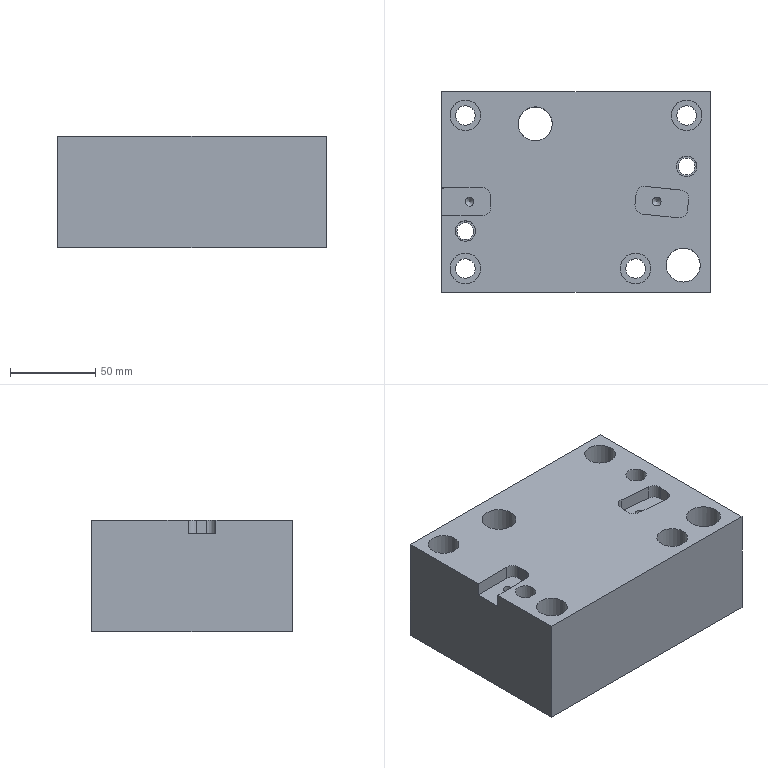Part | NX | features 23 2 | 1 solid | 45 faces | box 158 x 118 x 65.4 mm | volume 1108387 mm3 | cylinder 22 | plane 21 | cone 2 | commonest cylinder face diameters 10 x6 11.5 x4 18 x4 5.2 x2 10.001 x2 12 x2
STEP:
#1=CARTESIAN_POINT('',(1768.,-262.,2.4));
#2=VERTEX_POINT('',#1);
#3=CARTESIAN_POINT('',(1759.,-262.,2.4));
#4=DIRECTION('',(0.,0.,-1.));
#5=DIRECTION('',(1.,0.,0.));
#6=AXIS2_PLACEMENT_3D('',#3,#4,#5);
#7=CIRCLE('',#6,9.);
#8=EDGE_CURVE('',#2,#2,#7,.T.);
#9=ORIENTED_EDGE('',*,*,#8,.T.);
#10=EDGE_LOOP('',(#9));
#11=FACE_BOUND('',#10,.T.);
#12=CARTESIAN_POINT('',(1757.,-340.,2.4));
#13=VERTEX_POINT('',#12);
#14=CARTESIAN_POINT('',(1757.,-350.,2.4));
#15=DIRECTION('',(0.,-0.000000004,1.));
#16=DIRECTION('',(0.,1.,0.000000004));
#17=AXIS2_PLACEMENT_3D('',#14,#15,#16);
#18=CIRCLE('',#17,10.);
#19=EDGE_CURVE('',#13,#13,#18,.T.);
#20=ORIENTED_EDGE('',*,*,#19,.F.);
#21=EDGE_LOOP('',(#20));
#22=FACE_BOUND('',#21,.T.);
#23=CARTESIAN_POINT('',(1728.677,-314.602,2.4));
#24=VERTEX_POINT('',#23);
#25=CARTESIAN_POINT('',(1729.324,-308.234,2.4));
#26=VERTEX_POINT('',#25);
#27=CARTESIAN_POINT('',(1741.75,-185.905,2.4));
#28=DIRECTION('',(0.1011,0.9949,0.000000004));
#29=VECTOR('',#28,1000.);
#30=LINE('',#27,#29);
#31=EDGE_CURVE('',#24,#26,#30,.T.);
#32=ORIENTED_EDGE('',*,*,#31,.T.);
#33=CARTESIAN_POINT('',(1734.804,-303.765,2.4));
#34=VERTEX_POINT('',#33);
#35=CARTESIAN_POINT('',(1734.299,-308.74,2.4));
#36=DIRECTION('',(0.,0.000000004,-1.));
#37=DIRECTION('',(0.,1.,0.000000004));
#38=AXIS2_PLACEMENT_3D('',#35,#36,#37);
#39=CIRCLE('',#38,5.);
#40=EDGE_CURVE('',#26,#34,#39,.T.);
#41=ORIENTED_EDGE('',*,*,#40,.T.);
#42=CARTESIAN_POINT('',(1755.696,-305.887,2.4));
#43=VERTEX_POINT('',#42);
#44=CARTESIAN_POINT('',(1711.08,-301.355,2.4));
#45=DIRECTION('',(0.9949,-0.1011,0.));
#46=VECTOR('',#45,1000.);
#47=LINE('',#44,#46);
#48=EDGE_CURVE('',#34,#43,#47,.T.);
#49=ORIENTED_EDGE('',*,*,#48,.T.);
#50=CARTESIAN_POINT('',(1760.166,-311.367,2.4));
#51=VERTEX_POINT('',#50);
#52=CARTESIAN_POINT('',(1755.191,-310.862,2.4));
#53=DIRECTION('',(0.,0.000000004,-1.));
#54=DIRECTION('',(0.,1.,0.000000004));
#55=AXIS2_PLACEMENT_3D('',#52,#53,#54);
#56=CIRCLE('',#55,5.);
#57=EDGE_CURVE('',#43,#51,#56,.T.);
#58=ORIENTED_EDGE('',*,*,#57,.T.);
#59=CARTESIAN_POINT('',(1759.519,-317.734,2.4));
#60=VERTEX_POINT('',#59);
#61=CARTESIAN_POINT('',(1772.591,-189.037,2.4));
#62=DIRECTION('',(-0.1011,-0.9949,-0.000000004));
#63=VECTOR('',#62,1000.);
#64=LINE('',#61,#63);
#65=EDGE_CURVE('',#51,#60,#64,.T.);
#66=ORIENTED_EDGE('',*,*,#65,.T.);
#67=CARTESIAN_POINT('',(1754.039,-322.203,2.4));
#68=VERTEX_POINT('',#67);
#69=CARTESIAN_POINT('',(1754.544,-317.229,2.4));
#70=DIRECTION('',(0.,0.000000004,-1.));
#71=DIRECTION('',(0.,1.,0.000000004));
#72=AXIS2_PLACEMENT_3D('',#69,#70,#71);
#73=CIRCLE('',#72,5.);
#74=EDGE_CURVE('',#60,#68,#73,.T.);
#75=ORIENTED_EDGE('',*,*,#74,.T.);
#76=CARTESIAN_POINT('',(1733.147,-320.081,2.4));
#77=VERTEX_POINT('',#76);
#78=CARTESIAN_POINT('',(1709.422,-317.671,2.4));
#79=DIRECTION('',(-0.9949,0.1011,0.));
#80=VECTOR('',#79,1000.);
#81=LINE('',#78,#80);
#82=EDGE_CURVE('',#68,#77,#81,.T.);
#83=ORIENTED_EDGE('',*,*,#82,.T.);
#84=CARTESIAN_POINT('',(1733.652,-315.107,2.4));
#85=DIRECTION('',(0.,0.000000004,-1.));
#86=DIRECTION('',(0.,1.,0.000000004));
#87=AXIS2_PLACEMENT_3D('',#84,#85,#86);
#88=CIRCLE('',#87,5.);
#89=EDGE_CURVE('',#77,#24,#88,.T.);
#90=ORIENTED_EDGE('',*,*,#89,.T.);
#91=EDGE_LOOP('',(#32,#41,#49,#58,#66,#75,#83,#90));
#92=FACE_BOUND('',#91,.T.);
#93=CARTESIAN_POINT('',(1738.,-352.,2.4));
#94=VERTEX_POINT('',#93);
#95=CARTESIAN_POINT('',(1729.,-352.,2.4));
#96=DIRECTION('',(0.,0.,-1.));
#97=DIRECTION('',(1.,0.,0.));
#98=AXIS2_PLACEMENT_3D('',#95,#96,#97);
#99=CIRCLE('',#98,9.);
#100=EDGE_CURVE('',#94,#94,#99,.T.);
#101=ORIENTED_EDGE('',*,*,#100,.T.);
#102=EDGE_LOOP('',(#101));
#103=FACE_BOUND('',#102,.T.);
#104=CARTESIAN_POINT('',(1638.,-352.,2.4));
#105=VERTEX_POINT('',#104);
#106=CARTESIAN_POINT('',(1629.,-352.,2.4));
#107=DIRECTION('',(0.,0.,-1.));
#108=DIRECTION('',(1.,0.,0.));
#109=AXIS2_PLACEMENT_3D('',#106,#107,#108);
#110=CIRCLE('',#109,9.);
#111=EDGE_CURVE('',#105,#105,#110,.T.);
#112=ORIENTED_EDGE('',*,*,#111,.T.);
#113=EDGE_LOOP('',(#112));
#114=FACE_BOUND('',#113,.T.);
#115=CARTESIAN_POINT('',(1629.,-324.,2.4));
#116=VERTEX_POINT('',#115);
#117=CARTESIAN_POINT('',(1629.,-330.,2.4));
#118=DIRECTION('',(0.,0.000000004,-1.));
#119=DIRECTION('',(0.,1.,0.000000004));
#120=AXIS2_PLACEMENT_3D('',#117,#118,#119);
#121=CIRCLE('',#120,6.);
#122=EDGE_CURVE('',#116,#116,#121,.T.);
#123=ORIENTED_EDGE('',*,*,#122,.T.);
#124=EDGE_LOOP('',(#123));
#125=FACE_BOUND('',#124,.T.);
#126=CARTESIAN_POINT('',(1638.,-262.,2.4));
#127=VERTEX_POINT('',#126);
#128=CARTESIAN_POINT('',(1629.,-262.,2.4));
#129=DIRECTION('',(0.,0.,-1.));
#130=DIRECTION('',(1.,0.,0.));
#131=AXIS2_PLACEMENT_3D('',#128,#129,#130);
#132=CIRCLE('',#131,9.);
#133=EDGE_CURVE('',#127,#127,#132,.T.);
#134=ORIENTED_EDGE('',*,*,#133,.T.);
#135=EDGE_LOOP('',(#134));
#136=FACE_BOUND('',#135,.T.);
#137=CARTESIAN_POINT('',(1759.,-286.,2.4));
#138=VERTEX_POINT('',#137);
#139=CARTESIAN_POINT('',(1759.,-292.,2.4));
#140=DIRECTION('',(0.,0.000000004,-1.));
#141=DIRECTION('',(0.,1.,0.000000004));
#142=AXIS2_PLACEMENT_3D('',#139,#140,#141);
#143=CIRCLE('',#142,6.);
#144=EDGE_CURVE('',#138,#138,#143,.T.);
#145=ORIENTED_EDGE('',*,*,#144,.T.);
#146=EDGE_LOOP('',(#145));
#147=FACE_BOUND('',#146,.T.);
#148=CARTESIAN_POINT('',(1670.,-257.,2.4));
#149=VERTEX_POINT('',#148);
#150=CARTESIAN_POINT('',(1670.,-267.,2.4));
#151=DIRECTION('',(0.,0.000000004,-1.));
#152=DIRECTION('',(0.,1.,0.000000004));
#153=AXIS2_PLACEMENT_3D('',#150,#151,#152);
#154=CIRCLE('',#153,10.);
#155=EDGE_CURVE('',#149,#149,#154,.T.);
#156=ORIENTED_EDGE('',*,*,#155,.T.);
#157=EDGE_LOOP('',(#156));
#158=FACE_BOUND('',#157,.T.);
#159=CARTESIAN_POINT('',(1773.,-366.,2.4));
#160=VERTEX_POINT('',#159);
#161=CARTESIAN_POINT('',(1615.,-366.,2.4));
#162=VERTEX_POINT('',#161);
#163=CARTESIAN_POINT('',(1723.,-366.,2.4));
#164=DIRECTION('',(-1.,0.,0.));
#165=VECTOR('',#164,1000.);
#166=LINE('',#163,#165);
#167=EDGE_CURVE('',#160,#162,#166,.T.);
#168=ORIENTED_EDGE('',*,*,#167,.F.);
#169=CARTESIAN_POINT('',(1773.,-248.,2.4));
#170=VERTEX_POINT('',#169);
#171=CARTESIAN_POINT('',(1773.,-184.,2.4));
#172=DIRECTION('',(0.,-1.,-0.000000004));
#173=VECTOR('',#172,1000.);
#174=LINE('',#171,#173);
#175=EDGE_CURVE('',#170,#160,#174,.T.);
#176=ORIENTED_EDGE('',*,*,#175,.F.);
#177=CARTESIAN_POINT('',(1615.,-248.,2.4));
#178=VERTEX_POINT('',#177);
#179=CARTESIAN_POINT('',(1723.,-248.,2.4));
#180=DIRECTION('',(-1.,0.,0.));
#181=VECTOR('',#180,1000.);
#182=LINE('',#179,#181);
#183=EDGE_CURVE('',#170,#178,#182,.T.);
#184=ORIENTED_EDGE('',*,*,#183,.T.);
#185=CARTESIAN_POINT('',(1615.,-304.706,2.4));
#186=VERTEX_POINT('',#185);
#187=CARTESIAN_POINT('',(1615.,-184.,2.4));
#188=DIRECTION('',(0.,-1.,-0.000000004));
#189=VECTOR('',#188,1000.);
#190=LINE('',#187,#189);
#191=EDGE_CURVE('',#178,#186,#190,.T.);
#192=ORIENTED_EDGE('',*,*,#191,.T.);
#193=CARTESIAN_POINT('',(1638.846,-304.456,2.4));
#194=VERTEX_POINT('',#193);
#195=CARTESIAN_POINT('',(1724.252,-303.562,2.4));
#196=DIRECTION('',(0.9999,0.01047,0.));
#197=VECTOR('',#196,1000.);
#198=LINE('',#195,#197);
#199=EDGE_CURVE('',#186,#194,#198,.T.);
#200=ORIENTED_EDGE('',*,*,#199,.T.);
#201=CARTESIAN_POINT('',(1643.899,-309.404,2.4));
#202=VERTEX_POINT('',#201);
#203=CARTESIAN_POINT('',(1638.899,-309.456,2.4));
#204=DIRECTION('',(0.,0.000000004,-1.));
#205=DIRECTION('',(0.,1.,0.000000004));
#206=AXIS2_PLACEMENT_3D('',#203,#204,#205);
#207=CIRCLE('',#206,5.);
#208=EDGE_CURVE('',#194,#202,#207,.T.);
#209=ORIENTED_EDGE('',*,*,#208,.T.);
#210=CARTESIAN_POINT('',(1643.966,-315.803,2.4));
#211=VERTEX_POINT('',#210);
#212=CARTESIAN_POINT('',(1642.594,-184.842,2.4));
#213=DIRECTION('',(0.01047,-0.9999,-0.000000004));
#214=VECTOR('',#213,1000.);
#215=LINE('',#212,#214);
#216=EDGE_CURVE('',#202,#211,#215,.T.);
#217=ORIENTED_EDGE('',*,*,#216,.T.);
#218=CARTESIAN_POINT('',(1639.018,-320.855,2.4));
#219=VERTEX_POINT('',#218);
#220=CARTESIAN_POINT('',(1638.966,-315.856,2.4));
#221=DIRECTION('',(0.,0.000000004,-1.));
#222=DIRECTION('',(0.,1.,0.000000004));
#223=AXIS2_PLACEMENT_3D('',#220,#221,#222);
#224=CIRCLE('',#223,5.);
#225=EDGE_CURVE('',#211,#219,#224,.T.);
#226=ORIENTED_EDGE('',*,*,#225,.T.);
#227=CARTESIAN_POINT('',(1615.,-321.107,2.4));
#228=VERTEX_POINT('',#227);
#229=CARTESIAN_POINT('',(1724.424,-319.961,2.4));
#230=DIRECTION('',(-0.9999,-0.01047,0.));
#231=VECTOR('',#230,1000.);
#232=LINE('',#229,#231);
#233=EDGE_CURVE('',#219,#228,#232,.T.);
#234=ORIENTED_EDGE('',*,*,#233,.T.);
#235=CARTESIAN_POINT('',(1615.,-184.,2.4));
#236=DIRECTION('',(0.,-1.,-0.000000004));
#237=VECTOR('',#236,1000.);
#238=LINE('',#235,#237);
#239=EDGE_CURVE('',#228,#162,#238,.T.);
#240=ORIENTED_EDGE('',*,*,#239,.T.);
#241=EDGE_LOOP('',(#168,#176,#184,#192,#200,#209,#217,#226,#234,#240));
#242=FACE_BOUND('',#241,.T.);
#243=CARTESIAN_POINT('',(1723.,-184.,2.4));
#244=DIRECTION('',(0.,0.000000004,-1.));
#245=DIRECTION('',(0.,-1.,-0.000000004));
#246=AXIS2_PLACEMENT_3D('',#243,#244,#245);
#247=PLANE('',#246);
#248=ADVANCED_FACE('',(#11,#22,#92,#103,#114,#125,#136,#147,#158,#242),#247,.F.);
#249=CARTESIAN_POINT('',(1734.75,-352.,-63.));
#250=VERTEX_POINT('',#249);
#251=CARTESIAN_POINT('',(1729.,-352.,-63.));
#252=DIRECTION('',(0.,0.,1.));
#253=DIRECTION('',(1.,0.,0.));
#254=AXIS2_PLACEMENT_3D('',#251,#252,#253);
#255=CIRCLE('',#254,5.75);
#256=EDGE_CURVE('',#250,#250,#255,.T.);
#257=ORIENTED_EDGE('',*,*,#256,.T.);
#258=EDGE_LOOP('',(#257));
#259=FACE_BOUND('',#258,.T.);
#260=CARTESIAN_POINT('',(1634.75,-352.,-63.));
#261=VERTEX_POINT('',#260);
#262=CARTESIAN_POINT('',(1629.,-352.,-63.));
#263=DIRECTION('',(0.,0.,1.));
#264=DIRECTION('',(1.,0.,0.));
#265=AXIS2_PLACEMENT_3D('',#262,#263,#264);
#266=CIRCLE('',#265,5.75);
#267=EDGE_CURVE('',#261,#261,#266,.T.);
#268=ORIENTED_EDGE('',*,*,#267,.T.);
#269=EDGE_LOOP('',(#268));
#270=FACE_BOUND('',#269,.T.);
#271=CARTESIAN_POINT('',(1634.001,-330.,-63.));
#272=VERTEX_POINT('',#271);
#273=CARTESIAN_POINT('',(1629.,-330.,-63.));
#274=DIRECTION('',(0.,0.,1.));
#275=DIRECTION('',(1.,0.,0.));
#276=AXIS2_PLACEMENT_3D('',#273,#274,#275);
#277=CIRCLE('',#276,5.);
#278=EDGE_CURVE('',#272,#272,#277,.T.);
#279=ORIENTED_EDGE('',*,*,#278,.T.);
#280=EDGE_LOOP('',(#279));
#281=FACE_BOUND('',#280,.T.);
#282=CARTESIAN_POINT('',(1634.75,-262.,-63.));
#283=VERTEX_POINT('',#282);
#284=CARTESIAN_POINT('',(1629.,-262.,-63.));
#285=DIRECTION('',(0.,0.,1.));
#286=DIRECTION('',(1.,0.,0.));
#287=AXIS2_PLACEMENT_3D('',#284,#285,#286);
#288=CIRCLE('',#287,5.75);
#289=EDGE_CURVE('',#283,#283,#288,.T.);
#290=ORIENTED_EDGE('',*,*,#289,.T.);
#291=EDGE_LOOP('',(#290));
#292=FACE_BOUND('',#291,.T.);
#293=CARTESIAN_POINT('',(1764.001,-292.,-63.));
#294=VERTEX_POINT('',#293);
#295=CARTESIAN_POINT('',(1759.,-292.,-63.));
#296=DIRECTION('',(0.,0.,1.));
#297=DIRECTION('',(1.,0.,0.));
#298=AXIS2_PLACEMENT_3D('',#295,#296,#297);
#299=CIRCLE('',#298,5.);
#300=EDGE_CURVE('',#294,#294,#299,.T.);
#301=ORIENTED_EDGE('',*,*,#300,.T.);
#302=EDGE_LOOP('',(#301));
#303=FACE_BOUND('',#302,.T.);
#304=CARTESIAN_POINT('',(1764.75,-262.,-63.));
#305=VERTEX_POINT('',#304);
#306=CARTESIAN_POINT('',(1759.,-262.,-63.));
#307=DIRECTION('',(0.,0.,1.));
#308=DIRECTION('',(1.,0.,0.));
#309=AXIS2_PLACEMENT_3D('',#306,#307,#308);
#310=CIRCLE('',#309,5.75);
#311=EDGE_CURVE('',#305,#305,#310,.T.);
#312=ORIENTED_EDGE('',*,*,#311,.T.);
#313=EDGE_LOOP('',(#312));
#314=FACE_BOUND('',#313,.T.);
#315=CARTESIAN_POINT('',(1680.,-267.,-63.));
#316=VERTEX_POINT('',#315);
#317=CARTESIAN_POINT('',(1670.,-267.,-63.));
#318=DIRECTION('',(0.,0.,1.));
#319=DIRECTION('',(1.,0.,0.));
#320=AXIS2_PLACEMENT_3D('',#317,#318,#319);
#321=CIRCLE('',#320,10.);
#322=EDGE_CURVE('',#316,#316,#321,.T.);
#323=ORIENTED_EDGE('',*,*,#322,.T.);
#324=EDGE_LOOP('',(#323));
#325=FACE_BOUND('',#324,.T.);
#326=CARTESIAN_POINT('',(1615.,-366.,-63.));
#327=VERTEX_POINT('',#326);
#328=CARTESIAN_POINT('',(1615.,-248.,-63.));
#329=VERTEX_POINT('',#328);
#330=CARTESIAN_POINT('',(1615.,-184.,-63.));
#331=DIRECTION('',(0.,1.,0.));
#332=VECTOR('',#331,1000.);
#333=LINE('',#330,#332);
#334=EDGE_CURVE('',#327,#329,#333,.T.);
#335=ORIENTED_EDGE('',*,*,#334,.T.);
#336=CARTESIAN_POINT('',(1773.,-248.,-63.));
#337=VERTEX_POINT('',#336);
#338=CARTESIAN_POINT('',(1616.5,-248.,-63.));
#339=DIRECTION('',(-1.,0.,0.));
#340=VECTOR('',#339,1000.);
#341=LINE('',#338,#340);
#342=EDGE_CURVE('',#337,#329,#341,.T.);
#343=ORIENTED_EDGE('',*,*,#342,.F.);
#344=CARTESIAN_POINT('',(1773.,-366.,-63.));
#345=VERTEX_POINT('',#344);
#346=CARTESIAN_POINT('',(1773.,-184.,-63.));
#347=DIRECTION('',(0.,1.,0.));
#348=VECTOR('',#347,1000.);
#349=LINE('',#346,#348);
#350=EDGE_CURVE('',#345,#337,#349,.T.);
#351=ORIENTED_EDGE('',*,*,#350,.F.);
#352=CARTESIAN_POINT('',(1723.,-366.,-63.));
#353=DIRECTION('',(-1.,0.,0.));
#354=VECTOR('',#353,1000.);
#355=LINE('',#352,#354);
#356=EDGE_CURVE('',#345,#327,#355,.T.);
#357=ORIENTED_EDGE('',*,*,#356,.T.);
#358=EDGE_LOOP('',(#335,#343,#351,#357));
#359=FACE_BOUND('',#358,.T.);
#360=CARTESIAN_POINT('',(1767.,-350.,-63.));
#361=VERTEX_POINT('',#360);
#362=CARTESIAN_POINT('',(1757.,-350.,-63.));
#363=DIRECTION('',(0.,0.,1.));
#364=DIRECTION('',(1.,0.,0.));
#365=AXIS2_PLACEMENT_3D('',#362,#363,#364);
#366=CIRCLE('',#365,10.);
#367=EDGE_CURVE('',#361,#361,#366,.T.);
#368=ORIENTED_EDGE('',*,*,#367,.T.);
#369=EDGE_LOOP('',(#368));
#370=FACE_BOUND('',#369,.T.);
#371=CARTESIAN_POINT('',(1723.,-184.,-63.));
#372=DIRECTION('',(0.,0.,1.));
#373=DIRECTION('',(-1.,0.,0.));
#374=AXIS2_PLACEMENT_3D('',#371,#372,#373);
#375=PLANE('',#374);
#376=ADVANCED_FACE('',(#259,#270,#281,#292,#303,#314,#325,#359,#370),#375,.F.);
#377=CARTESIAN_POINT('',(1773.,-366.,0.));
#378=DIRECTION('',(0.,0.,1.));
#379=VECTOR('',#378,1000.);
#380=LINE('',#377,#379);
#381=EDGE_CURVE('',#345,#160,#380,.T.);
#382=ORIENTED_EDGE('',*,*,#381,.T.);
#383=ORIENTED_EDGE('',*,*,#167,.T.);
#384=CARTESIAN_POINT('',(1615.,-366.,0.));
#385=DIRECTION('',(0.,0.,1.));
#386=VECTOR('',#385,1000.);
#387=LINE('',#384,#386);
#388=EDGE_CURVE('',#327,#162,#387,.T.);
#389=ORIENTED_EDGE('',*,*,#388,.F.);
#390=ORIENTED_EDGE('',*,*,#356,.F.);
#391=EDGE_LOOP('',(#382,#383,#389,#390));
#392=FACE_BOUND('',#391,.T.);
#393=CARTESIAN_POINT('',(1723.,-366.,0.));
#394=DIRECTION('',(0.,-1.,0.));
#395=DIRECTION('',(0.,0.,1.));
#396=AXIS2_PLACEMENT_3D('',#393,#394,#395);
#397=PLANE('',#396);
#398=ADVANCED_FACE('',(#392),#397,.T.);
#399=ORIENTED_EDGE('',*,*,#239,.F.);
#400=CARTESIAN_POINT('',(1615.,-321.107,-5.6));
#401=VERTEX_POINT('',#400);
#402=CARTESIAN_POINT('',(1615.,-321.107,0.));
#403=DIRECTION('',(0.,0.,-1.));
#404=VECTOR('',#403,1000.);
#405=LINE('',#402,#404);
#406=EDGE_CURVE('',#228,#401,#405,.T.);
#407=ORIENTED_EDGE('',*,*,#406,.T.);
#408=CARTESIAN_POINT('',(1615.,-304.706,-5.6));
#409=VERTEX_POINT('',#408);
#410=CARTESIAN_POINT('',(1615.,-184.,-5.6));
#411=DIRECTION('',(0.,1.,0.));
#412=VECTOR('',#411,1000.);
#413=LINE('',#410,#412);
#414=EDGE_CURVE('',#401,#409,#413,.T.);
#415=ORIENTED_EDGE('',*,*,#414,.T.);
#416=CARTESIAN_POINT('',(1615.,-304.706,0.));
#417=DIRECTION('',(0.,0.,1.));
#418=VECTOR('',#417,1000.);
#419=LINE('',#416,#418);
#420=EDGE_CURVE('',#409,#186,#419,.T.);
#421=ORIENTED_EDGE('',*,*,#420,.T.);
#422=ORIENTED_EDGE('',*,*,#191,.F.);
#423=CARTESIAN_POINT('',(1615.,-248.,0.));
#424=DIRECTION('',(0.,0.,1.));
#425=VECTOR('',#424,1000.);
#426=LINE('',#423,#425);
#427=EDGE_CURVE('',#329,#178,#426,.T.);
#428=ORIENTED_EDGE('',*,*,#427,.F.);
#429=ORIENTED_EDGE('',*,*,#334,.F.);
#430=ORIENTED_EDGE('',*,*,#388,.T.);
#431=EDGE_LOOP('',(#399,#407,#415,#421,#422,#428,#429,#430));
#432=FACE_BOUND('',#431,.T.);
#433=CARTESIAN_POINT('',(1615.,-184.,0.));
#434=DIRECTION('',(1.,0.,0.));
#435=DIRECTION('',(0.,0.,1.));
#436=AXIS2_PLACEMENT_3D('',#433,#434,#435);
#437=PLANE('',#436);
#438=ADVANCED_FACE('',(#432),#437,.F.);
#439=CARTESIAN_POINT('',(1773.,-248.,0.));
#440=DIRECTION('',(0.,0.,1.));
#441=VECTOR('',#440,1000.);
#442=LINE('',#439,#441);
#443=EDGE_CURVE('',#337,#170,#442,.T.);
#444=ORIENTED_EDGE('',*,*,#443,.T.);
#445=ORIENTED_EDGE('',*,*,#175,.T.);
#446=ORIENTED_EDGE('',*,*,#381,.F.);
#447=ORIENTED_EDGE('',*,*,#350,.T.);
#448=EDGE_LOOP('',(#444,#445,#446,#447));
#449=FACE_BOUND('',#448,.T.);
#450=CARTESIAN_POINT('',(1773.,-184.,0.));
#451=DIRECTION('',(1.,0.,0.));
#452=DIRECTION('',(0.,0.,1.));
#453=AXIS2_PLACEMENT_3D('',#450,#451,#452);
#454=PLANE('',#453);
#455=ADVANCED_FACE('',(#449),#454,.T.);
#456=ORIENTED_EDGE('',*,*,#183,.F.);
#457=ORIENTED_EDGE('',*,*,#443,.F.);
#458=ORIENTED_EDGE('',*,*,#342,.T.);
#459=ORIENTED_EDGE('',*,*,#427,.T.);
#460=EDGE_LOOP('',(#456,#457,#458,#459));
#461=FACE_BOUND('',#460,.T.);
#462=CARTESIAN_POINT('',(1616.5,-248.,-55.3));
#463=DIRECTION('',(0.,-1.,0.));
#464=DIRECTION('',(0.,0.,1.));
#465=AXIS2_PLACEMENT_3D('',#462,#463,#464);
#466=PLANE('',#465);
#467=ADVANCED_FACE('',(#461),#466,.F.);
#468=ORIENTED_EDGE('',*,*,#322,.F.);
#469=EDGE_LOOP('',(#468));
#470=FACE_BOUND('',#469,.T.);
#471=ORIENTED_EDGE('',*,*,#155,.F.);
#472=EDGE_LOOP('',(#471));
#473=FACE_BOUND('',#472,.T.);
#474=CARTESIAN_POINT('',(1670.,-267.,-193.8));
#475=DIRECTION('',(0.,0.,1.));
#476=DIRECTION('',(-1.,0.,0.));
#477=AXIS2_PLACEMENT_3D('',#474,#475,#476);
#478=CYLINDRICAL_SURFACE('',#477,10.);
#479=ADVANCED_FACE('',(#470,#473),#478,.F.);
#480=ORIENTED_EDGE('',*,*,#367,.F.);
#481=EDGE_LOOP('',(#480));
#482=FACE_BOUND('',#481,.T.);
#483=ORIENTED_EDGE('',*,*,#19,.T.);
#484=EDGE_LOOP('',(#483));
#485=FACE_BOUND('',#484,.T.);
#486=CARTESIAN_POINT('',(1757.,-350.,-193.8));
#487=DIRECTION('',(0.,0.,1.));
#488=DIRECTION('',(-1.,0.,0.));
#489=AXIS2_PLACEMENT_3D('',#486,#487,#488);
#490=CYLINDRICAL_SURFACE('',#489,10.);
#491=ADVANCED_FACE('',(#482,#485),#490,.F.);
#492=CARTESIAN_POINT('',(1764.75,-262.,-33.));
#493=VERTEX_POINT('',#492);
#494=CARTESIAN_POINT('',(1759.,-262.,-33.));
#495=DIRECTION('',(0.,0.,-1.));
#496=DIRECTION('',(1.,0.,0.));
#497=AXIS2_PLACEMENT_3D('',#494,#495,#496);
#498=CIRCLE('',#497,5.75);
#499=EDGE_CURVE('',#493,#493,#498,.T.);
#500=ORIENTED_EDGE('',*,*,#499,.F.);
#501=EDGE_LOOP('',(#500));
#502=FACE_BOUND('',#501,.T.);
#503=ORIENTED_EDGE('',*,*,#311,.F.);
#504=EDGE_LOOP('',(#503));
#505=FACE_BOUND('',#504,.T.);
#506=CARTESIAN_POINT('',(1759.,-262.,7.4));
#507=DIRECTION('',(0.,0.,-1.));
#508=DIRECTION('',(-1.,0.,0.));
#509=AXIS2_PLACEMENT_3D('',#506,#507,#508);
#510=CYLINDRICAL_SURFACE('',#509,5.75);
#511=ADVANCED_FACE('',(#502,#505),#510,.F.);
#512=ORIENTED_EDGE('',*,*,#499,.T.);
#513=EDGE_LOOP('',(#512));
#514=FACE_BOUND('',#513,.T.);
#515=CARTESIAN_POINT('',(1768.,-262.,-33.));
#516=VERTEX_POINT('',#515);
#517=CARTESIAN_POINT('',(1759.,-262.,-33.));
#518=DIRECTION('',(0.,0.,-1.));
#519=DIRECTION('',(1.,0.,0.));
#520=AXIS2_PLACEMENT_3D('',#517,#518,#519);
#521=CIRCLE('',#520,9.);
#522=EDGE_CURVE('',#516,#516,#521,.T.);
#523=ORIENTED_EDGE('',*,*,#522,.F.);
#524=EDGE_LOOP('',(#523));
#525=FACE_BOUND('',#524,.T.);
#526=CARTESIAN_POINT('',(1759.,-262.,-33.));
#527=DIRECTION('',(0.,0.,-1.));
#528=DIRECTION('',(-1.,0.,0.));
#529=AXIS2_PLACEMENT_3D('',#526,#527,#528);
#530=PLANE('',#529);
#531=ADVANCED_FACE('',(#514,#525),#530,.F.);
#532=ORIENTED_EDGE('',*,*,#522,.T.);
#533=EDGE_LOOP('',(#532));
#534=FACE_BOUND('',#533,.T.);
#535=ORIENTED_EDGE('',*,*,#8,.F.);
#536=EDGE_LOOP('',(#535));
#537=FACE_BOUND('',#536,.T.);
#538=CARTESIAN_POINT('',(1759.,-262.,2.4));
#539=DIRECTION('',(0.,0.,-1.));
#540=DIRECTION('',(-1.,0.,0.));
#541=AXIS2_PLACEMENT_3D('',#538,#539,#540);
#542=CYLINDRICAL_SURFACE('',#541,9.);
#543=ADVANCED_FACE('',(#534,#537),#542,.F.);
#544=CARTESIAN_POINT('',(1765.,-292.,-34.));
#545=VERTEX_POINT('',#544);
#546=CARTESIAN_POINT('',(1759.,-292.,-34.));
#547=DIRECTION('',(0.,0.,-1.));
#548=DIRECTION('',(1.,0.,0.));
#549=AXIS2_PLACEMENT_3D('',#546,#547,#548);
#550=CIRCLE('',#549,6.);
#551=EDGE_CURVE('',#545,#545,#550,.T.);
#552=ORIENTED_EDGE('',*,*,#551,.T.);
#553=EDGE_LOOP('',(#552));
#554=FACE_BOUND('',#553,.T.);
#555=ORIENTED_EDGE('',*,*,#144,.F.);
#556=EDGE_LOOP('',(#555));
#557=FACE_BOUND('',#556,.T.);
#558=CARTESIAN_POINT('',(1759.,-292.,7.4));
#559=DIRECTION('',(0.,0.,-1.));
#560=DIRECTION('',(-1.,0.,0.));
#561=AXIS2_PLACEMENT_3D('',#558,#559,#560);
#562=CYLINDRICAL_SURFACE('',#561,6.);
#563=ADVANCED_FACE('',(#554,#557),#562,.F.);
#564=CARTESIAN_POINT('',(1764.001,-292.,-34.));
#565=VERTEX_POINT('',#564);
#566=CARTESIAN_POINT('',(1759.,-292.,-34.));
#567=DIRECTION('',(0.,0.,-1.));
#568=DIRECTION('',(1.,0.,0.));
#569=AXIS2_PLACEMENT_3D('',#566,#567,#568);
#570=CIRCLE('',#569,5.);
#571=EDGE_CURVE('',#565,#565,#570,.T.);
#572=ORIENTED_EDGE('',*,*,#571,.F.);
#573=EDGE_LOOP('',(#572));
#574=FACE_BOUND('',#573,.T.);
#575=ORIENTED_EDGE('',*,*,#300,.F.);
#576=EDGE_LOOP('',(#575));
#577=FACE_BOUND('',#576,.T.);
#578=CARTESIAN_POINT('',(1759.,-292.,7.4));
#579=DIRECTION('',(0.,0.,-1.));
#580=DIRECTION('',(-1.,0.,0.));
#581=AXIS2_PLACEMENT_3D('',#578,#579,#580);
#582=CYLINDRICAL_SURFACE('',#581,5.);
#583=ADVANCED_FACE('',(#574,#577),#582,.F.);
#584=ORIENTED_EDGE('',*,*,#571,.T.);
#585=EDGE_LOOP('',(#584));
#586=FACE_BOUND('',#585,.T.);
#587=ORIENTED_EDGE('',*,*,#551,.F.);
#588=EDGE_LOOP('',(#587));
#589=FACE_BOUND('',#588,.T.);
#590=CARTESIAN_POINT('',(1759.,-292.,-34.));
#591=DIRECTION('',(0.,0.,-1.));
#592=DIRECTION('',(-1.,0.,0.));
#593=AXIS2_PLACEMENT_3D('',#590,#591,#592);
#594=PLANE('',#593);
#595=ADVANCED_FACE('',(#586,#589),#594,.F.);
#596=CARTESIAN_POINT('',(1634.75,-262.,-33.));
#597=VERTEX_POINT('',#596);
#598=CARTESIAN_POINT('',(1629.,-262.,-33.));
#599=DIRECTION('',(0.,0.,-1.));
#600=DIRECTION('',(1.,0.,0.));
#601=AXIS2_PLACEMENT_3D('',#598,#599,#600);
#602=CIRCLE('',#601,5.75);
#603=EDGE_CURVE('',#597,#597,#602,.T.);
#604=ORIENTED_EDGE('',*,*,#603,.F.);
#605=EDGE_LOOP('',(#604));
#606=FACE_BOUND('',#605,.T.);
#607=ORIENTED_EDGE('',*,*,#289,.F.);
#608=EDGE_LOOP('',(#607));
#609=FACE_BOUND('',#608,.T.);
#610=CARTESIAN_POINT('',(1629.,-262.,7.4));
#611=DIRECTION('',(0.,0.,-1.));
#612=DIRECTION('',(-1.,0.,0.));
#613=AXIS2_PLACEMENT_3D('',#610,#611,#612);
#614=CYLINDRICAL_SURFACE('',#613,5.75);
#615=ADVANCED_FACE('',(#606,#609),#614,.F.);
#616=ORIENTED_EDGE('',*,*,#603,.T.);
#617=EDGE_LOOP('',(#616));
#618=FACE_BOUND('',#617,.T.);
#619=CARTESIAN_POINT('',(1638.,-262.,-33.));
#620=VERTEX_POINT('',#619);
#621=CARTESIAN_POINT('',(1629.,-262.,-33.));
#622=DIRECTION('',(0.,0.,-1.));
#623=DIRECTION('',(1.,0.,0.));
#624=AXIS2_PLACEMENT_3D('',#621,#622,#623);
#625=CIRCLE('',#624,9.);
#626=EDGE_CURVE('',#620,#620,#625,.T.);
#627=ORIENTED_EDGE('',*,*,#626,.F.);
#628=EDGE_LOOP('',(#627));
#629=FACE_BOUND('',#628,.T.);
#630=CARTESIAN_POINT('',(1629.,-262.,-33.));
#631=DIRECTION('',(0.,0.,-1.));
#632=DIRECTION('',(-1.,0.,0.));
#633=AXIS2_PLACEMENT_3D('',#630,#631,#632);
#634=PLANE('',#633);
#635=ADVANCED_FACE('',(#618,#629),#634,.F.);
#636=ORIENTED_EDGE('',*,*,#626,.T.);
#637=EDGE_LOOP('',(#636));
#638=FACE_BOUND('',#637,.T.);
#639=ORIENTED_EDGE('',*,*,#133,.F.);
#640=EDGE_LOOP('',(#639));
#641=FACE_BOUND('',#640,.T.);
#642=CARTESIAN_POINT('',(1629.,-262.,2.4));
#643=DIRECTION('',(0.,0.,-1.));
#644=DIRECTION('',(-1.,0.,0.));
#645=AXIS2_PLACEMENT_3D('',#642,#643,#644);
#646=CYLINDRICAL_SURFACE('',#645,9.);
#647=ADVANCED_FACE('',(#638,#641),#646,.F.);
#648=CARTESIAN_POINT('',(1635.,-330.,-34.));
#649=VERTEX_POINT('',#648);
#650=CARTESIAN_POINT('',(1629.,-330.,-34.));
#651=DIRECTION('',(0.,0.,-1.));
#652=DIRECTION('',(1.,0.,0.));
#653=AXIS2_PLACEMENT_3D('',#650,#651,#652);
#654=CIRCLE('',#653,6.);
#655=EDGE_CURVE('',#649,#649,#654,.T.);
#656=ORIENTED_EDGE('',*,*,#655,.T.);
#657=EDGE_LOOP('',(#656));
#658=FACE_BOUND('',#657,.T.);
#659=ORIENTED_EDGE('',*,*,#122,.F.);
#660=EDGE_LOOP('',(#659));
#661=FACE_BOUND('',#660,.T.);
#662=CARTESIAN_POINT('',(1629.,-330.,7.4));
#663=DIRECTION('',(0.,0.,-1.));
#664=DIRECTION('',(-1.,0.,0.));
#665=AXIS2_PLACEMENT_3D('',#662,#663,#664);
#666=CYLINDRICAL_SURFACE('',#665,6.);
#667=ADVANCED_FACE('',(#658,#661),#666,.F.);
#668=CARTESIAN_POINT('',(1634.001,-330.,-34.));
#669=VERTEX_POINT('',#668);
#670=CARTESIAN_POINT('',(1629.,-330.,-34.));
#671=DIRECTION('',(0.,0.,-1.));
#672=DIRECTION('',(1.,0.,0.));
#673=AXIS2_PLACEMENT_3D('',#670,#671,#672);
#674=CIRCLE('',#673,5.);
#675=EDGE_CURVE('',#669,#669,#674,.T.);
#676=ORIENTED_EDGE('',*,*,#675,.F.);
#677=EDGE_LOOP('',(#676));
#678=FACE_BOUND('',#677,.T.);
#679=ORIENTED_EDGE('',*,*,#278,.F.);
#680=EDGE_LOOP('',(#679));
#681=FACE_BOUND('',#680,.T.);
#682=CARTESIAN_POINT('',(1629.,-330.,7.4));
#683=DIRECTION('',(0.,0.,-1.));
#684=DIRECTION('',(-1.,0.,0.));
#685=AXIS2_PLACEMENT_3D('',#682,#683,#684);
#686=CYLINDRICAL_SURFACE('',#685,5.);
#687=ADVANCED_FACE('',(#678,#681),#686,.F.);
#688=ORIENTED_EDGE('',*,*,#675,.T.);
#689=EDGE_LOOP('',(#688));
#690=FACE_BOUND('',#689,.T.);
#691=ORIENTED_EDGE('',*,*,#655,.F.);
#692=EDGE_LOOP('',(#691));
#693=FACE_BOUND('',#692,.T.);
#694=CARTESIAN_POINT('',(1629.,-330.,-34.));
#695=DIRECTION('',(0.,0.,-1.));
#696=DIRECTION('',(-1.,0.,0.));
#697=AXIS2_PLACEMENT_3D('',#694,#695,#696);
#698=PLANE('',#697);
#699=ADVANCED_FACE('',(#690,#693),#698,.F.);
#700=CARTESIAN_POINT('',(1634.75,-352.,-33.));
#701=VERTEX_POINT('',#700);
#702=CARTESIAN_POINT('',(1629.,-352.,-33.));
#703=DIRECTION('',(0.,0.,-1.));
#704=DIRECTION('',(1.,0.,0.));
#705=AXIS2_PLACEMENT_3D('',#702,#703,#704);
#706=CIRCLE('',#705,5.75);
#707=EDGE_CURVE('',#701,#701,#706,.T.);
#708=ORIENTED_EDGE('',*,*,#707,.F.);
#709=EDGE_LOOP('',(#708));
#710=FACE_BOUND('',#709,.T.);
#711=ORIENTED_EDGE('',*,*,#267,.F.);
#712=EDGE_LOOP('',(#711));
#713=FACE_BOUND('',#712,.T.);
#714=CARTESIAN_POINT('',(1629.,-352.,7.4));
#715=DIRECTION('',(0.,0.,-1.));
#716=DIRECTION('',(-1.,0.,0.));
#717=AXIS2_PLACEMENT_3D('',#714,#715,#716);
#718=CYLINDRICAL_SURFACE('',#717,5.75);
#719=ADVANCED_FACE('',(#710,#713),#718,.F.);
#720=ORIENTED_EDGE('',*,*,#707,.T.);
#721=EDGE_LOOP('',(#720));
#722=FACE_BOUND('',#721,.T.);
#723=CARTESIAN_POINT('',(1638.,-352.,-33.));
#724=VERTEX_POINT('',#723);
#725=CARTESIAN_POINT('',(1629.,-352.,-33.));
#726=DIRECTION('',(0.,0.,-1.));
#727=DIRECTION('',(1.,0.,0.));
#728=AXIS2_PLACEMENT_3D('',#725,#726,#727);
#729=CIRCLE('',#728,9.);
#730=EDGE_CURVE('',#724,#724,#729,.T.);
#731=ORIENTED_EDGE('',*,*,#730,.F.);
#732=EDGE_LOOP('',(#731));
#733=FACE_BOUND('',#732,.T.);
#734=CARTESIAN_POINT('',(1629.,-352.,-33.));
#735=DIRECTION('',(0.,0.,-1.));
#736=DIRECTION('',(-1.,0.,0.));
#737=AXIS2_PLACEMENT_3D('',#734,#735,#736);
#738=PLANE('',#737);
#739=ADVANCED_FACE('',(#722,#733),#738,.F.);
#740=ORIENTED_EDGE('',*,*,#730,.T.);
#741=EDGE_LOOP('',(#740));
#742=FACE_BOUND('',#741,.T.);
#743=ORIENTED_EDGE('',*,*,#111,.F.);
#744=EDGE_LOOP('',(#743));
#745=FACE_BOUND('',#744,.T.);
#746=CARTESIAN_POINT('',(1629.,-352.,2.4));
#747=DIRECTION('',(0.,0.,-1.));
#748=DIRECTION('',(-1.,0.,0.));
#749=AXIS2_PLACEMENT_3D('',#746,#747,#748);
#750=CYLINDRICAL_SURFACE('',#749,9.);
#751=ADVANCED_FACE('',(#742,#745),#750,.F.);
#752=CARTESIAN_POINT('',(1734.75,-352.,-33.));
#753=VERTEX_POINT('',#752);
#754=CARTESIAN_POINT('',(1729.,-352.,-33.));
#755=DIRECTION('',(0.,0.,-1.));
#756=DIRECTION('',(1.,0.,0.));
#757=AXIS2_PLACEMENT_3D('',#754,#755,#756);
#758=CIRCLE('',#757,5.75);
#759=EDGE_CURVE('',#753,#753,#758,.T.);
#760=ORIENTED_EDGE('',*,*,#759,.F.);
#761=EDGE_LOOP('',(#760));
#762=FACE_BOUND('',#761,.T.);
#763=ORIENTED_EDGE('',*,*,#256,.F.);
#764=EDGE_LOOP('',(#763));
#765=FACE_BOUND('',#764,.T.);
#766=CARTESIAN_POINT('',(1729.,-352.,7.4));
#767=DIRECTION('',(0.,0.,-1.));
#768=DIRECTION('',(-1.,0.,0.));
#769=AXIS2_PLACEMENT_3D('',#766,#767,#768);
#770=CYLINDRICAL_SURFACE('',#769,5.75);
#771=ADVANCED_FACE('',(#762,#765),#770,.F.);
#772=ORIENTED_EDGE('',*,*,#759,.T.);
#773=EDGE_LOOP('',(#772));
#774=FACE_BOUND('',#773,.T.);
#775=CARTESIAN_POINT('',(1738.,-352.,-33.));
#776=VERTEX_POINT('',#775);
#777=CARTESIAN_POINT('',(1729.,-352.,-33.));
#778=DIRECTION('',(0.,0.,-1.));
#779=DIRECTION('',(1.,0.,0.));
#780=AXIS2_PLACEMENT_3D('',#777,#778,#779);
#781=CIRCLE('',#780,9.);
#782=EDGE_CURVE('',#776,#776,#781,.T.);
#783=ORIENTED_EDGE('',*,*,#782,.F.);
#784=EDGE_LOOP('',(#783));
#785=FACE_BOUND('',#784,.T.);
#786=CARTESIAN_POINT('',(1729.,-352.,-33.));
#787=DIRECTION('',(0.,0.,-1.));
#788=DIRECTION('',(-1.,0.,0.));
#789=AXIS2_PLACEMENT_3D('',#786,#787,#788);
#790=PLANE('',#789);
#791=ADVANCED_FACE('',(#774,#785),#790,.F.);
#792=ORIENTED_EDGE('',*,*,#782,.T.);
#793=EDGE_LOOP('',(#792));
#794=FACE_BOUND('',#793,.T.);
#795=ORIENTED_EDGE('',*,*,#100,.F.);
#796=EDGE_LOOP('',(#795));
#797=FACE_BOUND('',#796,.T.);
#798=CARTESIAN_POINT('',(1729.,-352.,2.4));
#799=DIRECTION('',(0.,0.,-1.));
#800=DIRECTION('',(-1.,0.,0.));
#801=AXIS2_PLACEMENT_3D('',#798,#799,#800);
#802=CYLINDRICAL_SURFACE('',#801,9.);
#803=ADVANCED_FACE('',(#794,#797),#802,.F.);
#804=CARTESIAN_POINT('',(1643.899,-309.404,-5.6));
#805=VERTEX_POINT('',#804);
#806=CARTESIAN_POINT('',(1643.899,-309.404,-5.6));
#807=DIRECTION('',(0.,0.,-1.));
#808=VECTOR('',#807,1000.);
#809=LINE('',#806,#808);
#810=EDGE_CURVE('',#202,#805,#809,.T.);
#811=ORIENTED_EDGE('',*,*,#810,.T.);
#812=CARTESIAN_POINT('',(1643.966,-315.803,-5.6));
#813=VERTEX_POINT('',#812);
#814=CARTESIAN_POINT('',(1643.932,-312.603,-5.6));
#815=DIRECTION('',(0.01047,-0.9999,0.));
#816=VECTOR('',#815,1000.);
#817=LINE('',#814,#816);
#818=EDGE_CURVE('',#805,#813,#817,.T.);
#819=ORIENTED_EDGE('',*,*,#818,.T.);
#820=CARTESIAN_POINT('',(1643.966,-315.803,-5.6));
#821=DIRECTION('',(0.,0.,1.));
#822=VECTOR('',#821,1000.);
#823=LINE('',#820,#822);
#824=EDGE_CURVE('',#813,#211,#823,.T.);
#825=ORIENTED_EDGE('',*,*,#824,.T.);
#826=ORIENTED_EDGE('',*,*,#216,.F.);
#827=EDGE_LOOP('',(#811,#819,#825,#826));
#828=FACE_BOUND('',#827,.T.);
#829=CARTESIAN_POINT('',(1643.932,-312.603,-5.6));
#830=DIRECTION('',(0.9999,0.01047,0.));
#831=DIRECTION('',(0.01047,-0.9999,0.));
#832=AXIS2_PLACEMENT_3D('',#829,#830,#831);
#833=PLANE('',#832);
#834=ADVANCED_FACE('',(#828),#833,.F.);
#835=CARTESIAN_POINT('',(1638.846,-304.456,-5.6));
#836=VERTEX_POINT('',#835);
#837=CARTESIAN_POINT('',(1638.846,-304.456,-5.6));
#838=DIRECTION('',(0.,0.,1.));
#839=VECTOR('',#838,1000.);
#840=LINE('',#837,#839);
#841=EDGE_CURVE('',#836,#194,#840,.T.);
#842=ORIENTED_EDGE('',*,*,#841,.F.);
#843=CARTESIAN_POINT('',(1638.899,-309.456,-5.6));
#844=DIRECTION('',(0.,0.,1.));
#845=DIRECTION('',(-1.,0.,0.));
#846=AXIS2_PLACEMENT_3D('',#843,#844,#845);
#847=CIRCLE('',#846,5.);
#848=EDGE_CURVE('',#805,#836,#847,.T.);
#849=ORIENTED_EDGE('',*,*,#848,.F.);
#850=ORIENTED_EDGE('',*,*,#810,.F.);
#851=ORIENTED_EDGE('',*,*,#208,.F.);
#852=EDGE_LOOP('',(#842,#849,#850,#851));
#853=FACE_BOUND('',#852,.T.);
#854=CARTESIAN_POINT('',(1638.899,-309.456,-5.6));
#855=DIRECTION('',(0.,0.,1.));
#856=DIRECTION('',(-1.,0.,0.));
#857=AXIS2_PLACEMENT_3D('',#854,#855,#856);
#858=CYLINDRICAL_SURFACE('',#857,5.);
#859=ADVANCED_FACE('',(#853),#858,.F.);
#860=ORIENTED_EDGE('',*,*,#824,.F.);
#861=CARTESIAN_POINT('',(1639.018,-320.855,-5.6));
#862=VERTEX_POINT('',#861);
#863=CARTESIAN_POINT('',(1638.966,-315.856,-5.6));
#864=DIRECTION('',(0.,0.,1.));
#865=DIRECTION('',(-1.,0.,0.));
#866=AXIS2_PLACEMENT_3D('',#863,#864,#865);
#867=CIRCLE('',#866,5.);
#868=EDGE_CURVE('',#862,#813,#867,.T.);
#869=ORIENTED_EDGE('',*,*,#868,.F.);
#870=CARTESIAN_POINT('',(1639.018,-320.855,-5.6));
#871=DIRECTION('',(0.,0.,-1.));
#872=VECTOR('',#871,1000.);
#873=LINE('',#870,#872);
#874=EDGE_CURVE('',#219,#862,#873,.T.);
#875=ORIENTED_EDGE('',*,*,#874,.F.);
#876=ORIENTED_EDGE('',*,*,#225,.F.);
#877=EDGE_LOOP('',(#860,#869,#875,#876));
#878=FACE_BOUND('',#877,.T.);
#879=CARTESIAN_POINT('',(1638.966,-315.856,-5.6));
#880=DIRECTION('',(0.,0.,1.));
#881=DIRECTION('',(-1.,0.,0.));
#882=AXIS2_PLACEMENT_3D('',#879,#880,#881);
#883=CYLINDRICAL_SURFACE('',#882,5.);
#884=ADVANCED_FACE('',(#878),#883,.F.);
#885=ORIENTED_EDGE('',*,*,#874,.T.);
#886=CARTESIAN_POINT('',(1628.519,-320.965,-5.6));
#887=DIRECTION('',(-0.9999,-0.01047,0.));
#888=VECTOR('',#887,1000.);
#889=LINE('',#886,#888);
#890=EDGE_CURVE('',#862,#401,#889,.T.);
#891=ORIENTED_EDGE('',*,*,#890,.T.);
#892=ORIENTED_EDGE('',*,*,#406,.F.);
#893=ORIENTED_EDGE('',*,*,#233,.F.);
#894=EDGE_LOOP('',(#885,#891,#892,#893));
#895=FACE_BOUND('',#894,.T.);
#896=CARTESIAN_POINT('',(1628.519,-320.965,-5.6));
#897=DIRECTION('',(0.01047,-0.9999,0.));
#898=DIRECTION('',(-0.9999,-0.01047,0.));
#899=AXIS2_PLACEMENT_3D('',#896,#897,#898);
#900=PLANE('',#899);
#901=ADVANCED_FACE('',(#895),#900,.F.);
#902=ORIENTED_EDGE('',*,*,#420,.F.);
#903=CARTESIAN_POINT('',(1628.347,-304.566,-5.6));
#904=DIRECTION('',(0.9999,0.01047,0.));
#905=VECTOR('',#904,1000.);
#906=LINE('',#903,#905);
#907=EDGE_CURVE('',#409,#836,#906,.T.);
#908=ORIENTED_EDGE('',*,*,#907,.T.);
#909=ORIENTED_EDGE('',*,*,#841,.T.);
#910=ORIENTED_EDGE('',*,*,#199,.F.);
#911=EDGE_LOOP('',(#902,#908,#909,#910));
#912=FACE_BOUND('',#911,.T.);
#913=CARTESIAN_POINT('',(1628.347,-304.566,-5.6));
#914=DIRECTION('',(-0.01047,0.9999,0.));
#915=DIRECTION('',(0.9999,0.01047,0.));
#916=AXIS2_PLACEMENT_3D('',#913,#914,#915);
#917=PLANE('',#916);
#918=ADVANCED_FACE('',(#912),#917,.F.);
#919=CARTESIAN_POINT('',(1634.033,-312.734,-5.6));
#920=VERTEX_POINT('',#919);
#921=CARTESIAN_POINT('',(1631.433,-312.734,-5.6));
#922=DIRECTION('',(0.,0.,-1.));
#923=DIRECTION('',(1.,0.,0.));
#924=AXIS2_PLACEMENT_3D('',#921,#922,#923);
#925=CIRCLE('',#924,2.6);
#926=EDGE_CURVE('',#920,#920,#925,.T.);
#927=ORIENTED_EDGE('',*,*,#926,.T.);
#928=EDGE_LOOP('',(#927));
#929=FACE_BOUND('',#928,.T.);
#930=ORIENTED_EDGE('',*,*,#890,.F.);
#931=ORIENTED_EDGE('',*,*,#868,.T.);
#932=ORIENTED_EDGE('',*,*,#818,.F.);
#933=ORIENTED_EDGE('',*,*,#848,.T.);
#934=ORIENTED_EDGE('',*,*,#907,.F.);
#935=ORIENTED_EDGE('',*,*,#414,.F.);
#936=EDGE_LOOP('',(#930,#931,#932,#933,#934,#935));
#937=FACE_BOUND('',#936,.T.);
#938=CARTESIAN_POINT('',(1628.433,-312.766,-5.6));
#939=DIRECTION('',(0.,0.,-1.));
#940=DIRECTION('',(1.,0.,0.));
#941=AXIS2_PLACEMENT_3D('',#938,#939,#940);
#942=PLANE('',#941);
#943=ADVANCED_FACE('',(#929,#937),#942,.F.);
#944=CARTESIAN_POINT('',(1754.039,-322.203,-5.6));
#945=VERTEX_POINT('',#944);
#946=CARTESIAN_POINT('',(1754.039,-322.203,-5.6));
#947=DIRECTION('',(0.,0.,-1.));
#948=VECTOR('',#947,1000.);
#949=LINE('',#946,#948);
#950=EDGE_CURVE('',#68,#945,#949,.T.);
#951=ORIENTED_EDGE('',*,*,#950,.T.);
#952=CARTESIAN_POINT('',(1733.147,-320.081,-5.6));
#953=VERTEX_POINT('',#952);
#954=CARTESIAN_POINT('',(1741.802,-320.96,-5.6));
#955=DIRECTION('',(-0.9949,0.1011,0.));
#956=VECTOR('',#955,1000.);
#957=LINE('',#954,#956);
#958=EDGE_CURVE('',#945,#953,#957,.T.);
#959=ORIENTED_EDGE('',*,*,#958,.T.);
#960=CARTESIAN_POINT('',(1733.147,-320.081,-5.6));
#961=DIRECTION('',(0.,0.,1.));
#962=VECTOR('',#961,1000.);
#963=LINE('',#960,#962);
#964=EDGE_CURVE('',#953,#77,#963,.T.);
#965=ORIENTED_EDGE('',*,*,#964,.T.);
#966=ORIENTED_EDGE('',*,*,#82,.F.);
#967=EDGE_LOOP('',(#951,#959,#965,#966));
#968=FACE_BOUND('',#967,.T.);
#969=CARTESIAN_POINT('',(1741.802,-320.96,-5.6));
#970=DIRECTION('',(-0.1011,-0.9949,0.));
#971=DIRECTION('',(-0.9949,0.1011,0.));
#972=AXIS2_PLACEMENT_3D('',#969,#970,#971);
#973=PLANE('',#972);
#974=ADVANCED_FACE('',(#968),#973,.F.);
#975=CARTESIAN_POINT('',(1728.677,-314.602,-5.6));
#976=VERTEX_POINT('',#975);
#977=CARTESIAN_POINT('',(1728.677,-314.602,-5.6));
#978=DIRECTION('',(0.,0.,-1.));
#979=VECTOR('',#978,1000.);
#980=LINE('',#977,#979);
#981=EDGE_CURVE('',#24,#976,#980,.T.);
#982=ORIENTED_EDGE('',*,*,#981,.T.);
#983=CARTESIAN_POINT('',(1729.324,-308.234,-5.6));
#984=VERTEX_POINT('',#983);
#985=CARTESIAN_POINT('',(1729.001,-311.418,-5.6));
#986=DIRECTION('',(0.1011,0.9949,0.));
#987=VECTOR('',#986,1000.);
#988=LINE('',#985,#987);
#989=EDGE_CURVE('',#976,#984,#988,.T.);
#990=ORIENTED_EDGE('',*,*,#989,.T.);
#991=CARTESIAN_POINT('',(1729.324,-308.234,-5.6));
#992=DIRECTION('',(0.,0.,1.));
#993=VECTOR('',#992,1000.);
#994=LINE('',#991,#993);
#995=EDGE_CURVE('',#984,#26,#994,.T.);
#996=ORIENTED_EDGE('',*,*,#995,.T.);
#997=ORIENTED_EDGE('',*,*,#31,.F.);
#998=EDGE_LOOP('',(#982,#990,#996,#997));
#999=FACE_BOUND('',#998,.T.);
#1000=CARTESIAN_POINT('',(1729.001,-311.418,-5.6));
#1001=DIRECTION('',(-0.9949,0.1011,0.));
#1002=DIRECTION('',(0.1011,0.9949,0.));
#1003=AXIS2_PLACEMENT_3D('',#1000,#1001,#1002);
#1004=PLANE('',#1003);
#1005=ADVANCED_FACE('',(#999),#1004,.F.);
#1006=CARTESIAN_POINT('',(1734.804,-303.765,-5.6));
#1007=VERTEX_POINT('',#1006);
#1008=CARTESIAN_POINT('',(1734.804,-303.765,-5.6));
#1009=DIRECTION('',(0.,0.,-1.));
#1010=VECTOR('',#1009,1000.);
#1011=LINE('',#1008,#1010);
#1012=EDGE_CURVE('',#34,#1007,#1011,.T.);
#1013=ORIENTED_EDGE('',*,*,#1012,.T.);
#1014=CARTESIAN_POINT('',(1755.696,-305.887,-5.6));
#1015=VERTEX_POINT('',#1014);
#1016=CARTESIAN_POINT('',(1743.459,-304.644,-5.6));
#1017=DIRECTION('',(0.9949,-0.1011,0.));
#1018=VECTOR('',#1017,1000.);
#1019=LINE('',#1016,#1018);
#1020=EDGE_CURVE('',#1007,#1015,#1019,.T.);
#1021=ORIENTED_EDGE('',*,*,#1020,.T.);
#1022=CARTESIAN_POINT('',(1755.696,-305.887,-5.6));
#1023=DIRECTION('',(0.,0.,1.));
#1024=VECTOR('',#1023,1000.);
#1025=LINE('',#1022,#1024);
#1026=EDGE_CURVE('',#1015,#43,#1025,.T.);
#1027=ORIENTED_EDGE('',*,*,#1026,.T.);
#1028=ORIENTED_EDGE('',*,*,#48,.F.);
#1029=EDGE_LOOP('',(#1013,#1021,#1027,#1028));
#1030=FACE_BOUND('',#1029,.T.);
#1031=CARTESIAN_POINT('',(1743.459,-304.644,-5.6));
#1032=DIRECTION('',(0.1011,0.9949,0.));
#1033=DIRECTION('',(0.9949,-0.1011,0.));
#1034=AXIS2_PLACEMENT_3D('',#1031,#1032,#1033);
#1035=PLANE('',#1034);
#1036=ADVANCED_FACE('',(#1030),#1035,.F.);
#1037=CARTESIAN_POINT('',(1760.166,-311.367,-5.6));
#1038=VERTEX_POINT('',#1037);
#1039=CARTESIAN_POINT('',(1760.166,-311.367,-5.6));
#1040=DIRECTION('',(0.,0.,-1.));
#1041=VECTOR('',#1040,1000.);
#1042=LINE('',#1039,#1041);
#1043=EDGE_CURVE('',#51,#1038,#1042,.T.);
#1044=ORIENTED_EDGE('',*,*,#1043,.T.);
#1045=CARTESIAN_POINT('',(1759.519,-317.734,-5.6));
#1046=VERTEX_POINT('',#1045);
#1047=CARTESIAN_POINT('',(1759.842,-314.551,-5.6));
#1048=DIRECTION('',(-0.1011,-0.9949,0.));
#1049=VECTOR('',#1048,1000.);
#1050=LINE('',#1047,#1049);
#1051=EDGE_CURVE('',#1038,#1046,#1050,.T.);
#1052=ORIENTED_EDGE('',*,*,#1051,.T.);
#1053=CARTESIAN_POINT('',(1759.519,-317.734,-5.6));
#1054=DIRECTION('',(0.,0.,1.));
#1055=VECTOR('',#1054,1000.);
#1056=LINE('',#1053,#1055);
#1057=EDGE_CURVE('',#1046,#60,#1056,.T.);
#1058=ORIENTED_EDGE('',*,*,#1057,.T.);
#1059=ORIENTED_EDGE('',*,*,#65,.F.);
#1060=EDGE_LOOP('',(#1044,#1052,#1058,#1059));
#1061=FACE_BOUND('',#1060,.T.);
#1062=CARTESIAN_POINT('',(1759.842,-314.551,-5.6));
#1063=DIRECTION('',(0.9949,-0.1011,0.));
#1064=DIRECTION('',(-0.1011,-0.9949,0.));
#1065=AXIS2_PLACEMENT_3D('',#1062,#1063,#1064);
#1066=PLANE('',#1065);
#1067=ADVANCED_FACE('',(#1061),#1066,.F.);
#1068=ORIENTED_EDGE('',*,*,#1026,.F.);
#1069=CARTESIAN_POINT('',(1755.191,-310.862,-5.6));
#1070=DIRECTION('',(0.,0.,1.));
#1071=DIRECTION('',(-1.,0.,0.));
#1072=AXIS2_PLACEMENT_3D('',#1069,#1070,#1071);
#1073=CIRCLE('',#1072,5.);
#1074=EDGE_CURVE('',#1038,#1015,#1073,.T.);
#1075=ORIENTED_EDGE('',*,*,#1074,.F.);
#1076=ORIENTED_EDGE('',*,*,#1043,.F.);
#1077=ORIENTED_EDGE('',*,*,#57,.F.);
#1078=EDGE_LOOP('',(#1068,#1075,#1076,#1077));
#1079=FACE_BOUND('',#1078,.T.);
#1080=CARTESIAN_POINT('',(1755.191,-310.862,-5.6));
#1081=DIRECTION('',(0.,0.,1.));
#1082=DIRECTION('',(-1.,0.,0.));
#1083=AXIS2_PLACEMENT_3D('',#1080,#1081,#1082);
#1084=CYLINDRICAL_SURFACE('',#1083,5.);
#1085=ADVANCED_FACE('',(#1079),#1084,.F.);
#1086=ORIENTED_EDGE('',*,*,#995,.F.);
#1087=CARTESIAN_POINT('',(1734.299,-308.74,-5.6));
#1088=DIRECTION('',(0.,0.,1.));
#1089=DIRECTION('',(-1.,0.,0.));
#1090=AXIS2_PLACEMENT_3D('',#1087,#1088,#1089);
#1091=CIRCLE('',#1090,5.);
#1092=EDGE_CURVE('',#1007,#984,#1091,.T.);
#1093=ORIENTED_EDGE('',*,*,#1092,.F.);
#1094=ORIENTED_EDGE('',*,*,#1012,.F.);
#1095=ORIENTED_EDGE('',*,*,#40,.F.);
#1096=EDGE_LOOP('',(#1086,#1093,#1094,#1095));
#1097=FACE_BOUND('',#1096,.T.);
#1098=CARTESIAN_POINT('',(1734.299,-308.74,-5.6));
#1099=DIRECTION('',(0.,0.,1.));
#1100=DIRECTION('',(-1.,0.,0.));
#1101=AXIS2_PLACEMENT_3D('',#1098,#1099,#1100);
#1102=CYLINDRICAL_SURFACE('',#1101,5.);
#1103=ADVANCED_FACE('',(#1097),#1102,.F.);
#1104=ORIENTED_EDGE('',*,*,#964,.F.);
#1105=CARTESIAN_POINT('',(1733.652,-315.107,-5.6));
#1106=DIRECTION('',(0.,0.,1.));
#1107=DIRECTION('',(-1.,0.,0.));
#1108=AXIS2_PLACEMENT_3D('',#1105,#1106,#1107);
#1109=CIRCLE('',#1108,5.);
#1110=EDGE_CURVE('',#976,#953,#1109,.T.);
#1111=ORIENTED_EDGE('',*,*,#1110,.F.);
#1112=ORIENTED_EDGE('',*,*,#981,.F.);
#1113=ORIENTED_EDGE('',*,*,#89,.F.);
#1114=EDGE_LOOP('',(#1104,#1111,#1112,#1113));
#1115=FACE_BOUND('',#1114,.T.);
#1116=CARTESIAN_POINT('',(1733.652,-315.107,-5.6));
#1117=DIRECTION('',(0.,0.,1.));
#1118=DIRECTION('',(-1.,0.,0.));
#1119=AXIS2_PLACEMENT_3D('',#1116,#1117,#1118);
#1120=CYLINDRICAL_SURFACE('',#1119,5.);
#1121=ADVANCED_FACE('',(#1115),#1120,.F.);
#1122=ORIENTED_EDGE('',*,*,#1057,.F.);
#1123=CARTESIAN_POINT('',(1754.544,-317.229,-5.6));
#1124=DIRECTION('',(0.,0.,1.));
#1125=DIRECTION('',(-1.,0.,0.));
#1126=AXIS2_PLACEMENT_3D('',#1123,#1124,#1125);
#1127=CIRCLE('',#1126,5.);
#1128=EDGE_CURVE('',#945,#1046,#1127,.T.);
#1129=ORIENTED_EDGE('',*,*,#1128,.F.);
#1130=ORIENTED_EDGE('',*,*,#950,.F.);
#1131=ORIENTED_EDGE('',*,*,#74,.F.);
#1132=EDGE_LOOP('',(#1122,#1129,#1130,#1131));
#1133=FACE_BOUND('',#1132,.T.);
#1134=CARTESIAN_POINT('',(1754.544,-317.229,-5.6));
#1135=DIRECTION('',(0.,0.,1.));
#1136=DIRECTION('',(-1.,0.,0.));
#1137=AXIS2_PLACEMENT_3D('',#1134,#1135,#1136);
#1138=CYLINDRICAL_SURFACE('',#1137,5.);
#1139=ADVANCED_FACE('',(#1133),#1138,.F.);
#1140=CARTESIAN_POINT('',(1744.037,-312.681,-5.6));
#1141=VERTEX_POINT('',#1140);
#1142=CARTESIAN_POINT('',(1741.437,-312.681,-5.6));
#1143=DIRECTION('',(0.,0.,-1.));
#1144=DIRECTION('',(1.,0.,0.));
#1145=AXIS2_PLACEMENT_3D('',#1142,#1143,#1144);
#1146=CIRCLE('',#1145,2.6);
#1147=EDGE_CURVE('',#1141,#1141,#1146,.T.);
#1148=ORIENTED_EDGE('',*,*,#1147,.T.);
#1149=EDGE_LOOP('',(#1148));
#1150=FACE_BOUND('',#1149,.T.);
#1151=ORIENTED_EDGE('',*,*,#1020,.F.);
#1152=ORIENTED_EDGE('',*,*,#1092,.T.);
#1153=ORIENTED_EDGE('',*,*,#989,.F.);
#1154=ORIENTED_EDGE('',*,*,#1110,.T.);
#1155=ORIENTED_EDGE('',*,*,#958,.F.);
#1156=ORIENTED_EDGE('',*,*,#1128,.T.);
#1157=ORIENTED_EDGE('',*,*,#1051,.F.);
#1158=ORIENTED_EDGE('',*,*,#1074,.T.);
#1159=EDGE_LOOP('',(#1151,#1152,#1153,#1154,#1155,#1156,#1157,#1158));
#1160=FACE_BOUND('',#1159,.T.);
#1161=CARTESIAN_POINT('',(1742.631,-312.802,-5.6));
#1162=DIRECTION('',(0.,0.,-1.));
#1163=DIRECTION('',(1.,0.,0.));
#1164=AXIS2_PLACEMENT_3D('',#1161,#1162,#1163);
#1165=PLANE('',#1164);
#1166=ADVANCED_FACE('',(#1150,#1160),#1165,.F.);
#1167=CARTESIAN_POINT('',(1628.833,-312.734,-27.));
#1168=VERTEX_POINT('',#1167);
#1169=CARTESIAN_POINT('',(1631.433,-312.734,-27.));
#1170=DIRECTION('',(0.,0.,-1.));
#1171=DIRECTION('',(-1.,0.,0.));
#1172=AXIS2_PLACEMENT_3D('',#1169,#1170,#1171);
#1173=CIRCLE('',#1172,2.6);
#1174=EDGE_CURVE('',#1168,#1168,#1173,.T.);
#1175=ORIENTED_EDGE('',*,*,#1174,.T.);
#1176=EDGE_LOOP('',(#1175));
#1177=FACE_BOUND('',#1176,.T.);
#1178=ORIENTED_EDGE('',*,*,#926,.F.);
#1179=EDGE_LOOP('',(#1178));
#1180=FACE_BOUND('',#1179,.T.);
#1181=CARTESIAN_POINT('',(1631.433,-312.734,-5.6));
#1182=DIRECTION('',(0.,0.,-1.));
#1183=DIRECTION('',(-1.,0.,0.));
#1184=AXIS2_PLACEMENT_3D('',#1181,#1182,#1183);
#1185=CYLINDRICAL_SURFACE('',#1184,2.6);
#1186=ADVANCED_FACE('',(#1177,#1180),#1185,.F.);
#1187=CARTESIAN_POINT('',(1631.433,-312.734,-29.6));
#1188=VERTEX_POINT('',#1187);
#1189=VERTEX_LOOP('',#1188);
#1190=FACE_BOUND('',#1189,.T.);
#1191=ORIENTED_EDGE('',*,*,#1174,.F.);
#1192=EDGE_LOOP('',(#1191));
#1193=FACE_BOUND('',#1192,.T.);
#1194=CARTESIAN_POINT('',(1631.433,-312.734,-27.));
#1195=DIRECTION('',(0.,0.,1.));
#1196=DIRECTION('',(-1.,0.,0.));
#1197=AXIS2_PLACEMENT_3D('',#1194,#1195,#1196);
#1198=CONICAL_SURFACE('',#1197,2.6,0.7854);
#1199=ADVANCED_FACE('',(#1190,#1193),#1198,.F.);
#1200=CARTESIAN_POINT('',(1738.837,-312.681,-27.));
#1201=VERTEX_POINT('',#1200);
#1202=CARTESIAN_POINT('',(1741.437,-312.681,-27.));
#1203=DIRECTION('',(0.,0.,-1.));
#1204=DIRECTION('',(-1.,0.,0.));
#1205=AXIS2_PLACEMENT_3D('',#1202,#1203,#1204);
#1206=CIRCLE('',#1205,2.6);
#1207=EDGE_CURVE('',#1201,#1201,#1206,.T.);
#1208=ORIENTED_EDGE('',*,*,#1207,.T.);
#1209=EDGE_LOOP('',(#1208));
#1210=FACE_BOUND('',#1209,.T.);
#1211=ORIENTED_EDGE('',*,*,#1147,.F.);
#1212=EDGE_LOOP('',(#1211));
#1213=FACE_BOUND('',#1212,.T.);
#1214=CARTESIAN_POINT('',(1741.437,-312.681,-5.6));
#1215=DIRECTION('',(0.,0.,-1.));
#1216=DIRECTION('',(-1.,0.,0.));
#1217=AXIS2_PLACEMENT_3D('',#1214,#1215,#1216);
#1218=CYLINDRICAL_SURFACE('',#1217,2.6);
#1219=ADVANCED_FACE('',(#1210,#1213),#1218,.F.);
#1220=CARTESIAN_POINT('',(1741.437,-312.681,-29.6));
#1221=VERTEX_POINT('',#1220);
#1222=VERTEX_LOOP('',#1221);
#1223=FACE_BOUND('',#1222,.T.);
#1224=ORIENTED_EDGE('',*,*,#1207,.F.);
#1225=EDGE_LOOP('',(#1224));
#1226=FACE_BOUND('',#1225,.T.);
#1227=CARTESIAN_POINT('',(1741.437,-312.681,-27.));
#1228=DIRECTION('',(0.,0.,1.));
#1229=DIRECTION('',(-1.,0.,0.));
#1230=AXIS2_PLACEMENT_3D('',#1227,#1228,#1229);
#1231=CONICAL_SURFACE('',#1230,2.6,0.7854);
#1232=ADVANCED_FACE('',(#1223,#1226),#1231,.F.);
#1233=CLOSED_SHELL('',(#248,#376,#398,#438,#455,#467,#479,#491,#511,#531,#543,#563,#583,#595,#615,#635,#647,#667,#687,#699,#719,#739,#751,#771,#791,#803,#834,#859,#884,#901,#918,#943,#974,#1005,#1036,#1067,#1085,#1103,#1121,#1139,#1166,#1186,#1199,#1219,#1232));
#1234=MANIFOLD_SOLID_BREP('',#1233);
#1235=(LENGTH_UNIT()NAMED_UNIT(*)SI_UNIT(.MILLI.,.METRE.));
#1236=UNCERTAINTY_MEASURE_WITH_UNIT(LENGTH_MEASURE(0.00001),#1235,'','');
#1237=(NAMED_UNIT(*)PLANE_ANGLE_UNIT()SI_UNIT($,.RADIAN.));
#1238=(NAMED_UNIT(*)SI_UNIT($,.STERADIAN.)SOLID_ANGLE_UNIT());
#1239=(GEOMETRIC_REPRESENTATION_CONTEXT(3)GLOBAL_UNCERTAINTY_ASSIGNED_CONTEXT((#1236))GLOBAL_UNIT_ASSIGNED_CONTEXT((#1235,#1237,#1238))REPRESENTATION_CONTEXT('',''));
#1240=ADVANCED_BREP_SHAPE_REPRESENTATION('',(#1234),#1239);